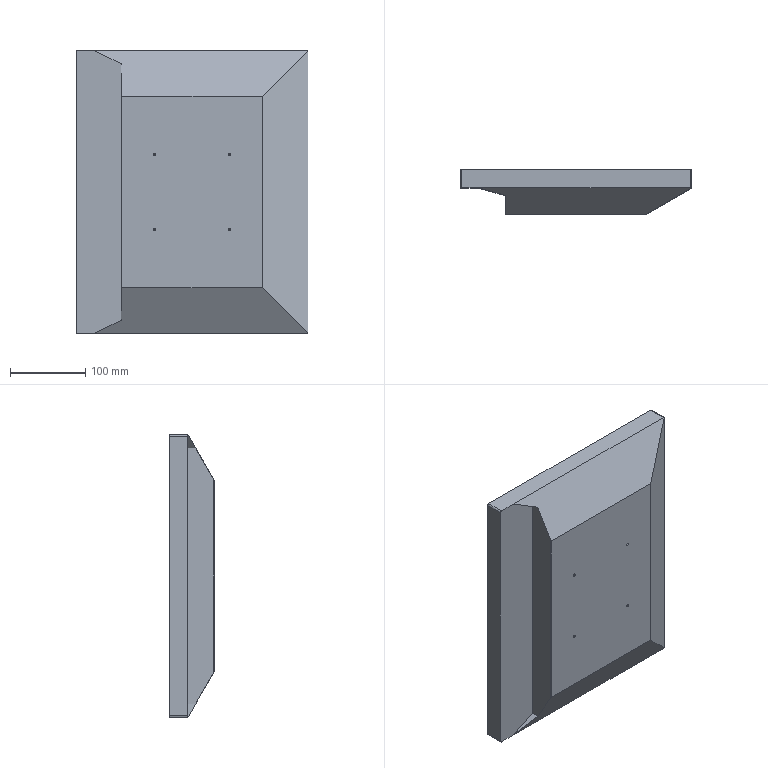Part | STEP file | E1715S | 1 solid | 253 faces | box 307.9 x 59 x 375.5 mm | volume 5016413 mm3 | plane 233 | cylinder 12 | cone 8 | commonest cylinder face diameters 3.3 x8 4 x4